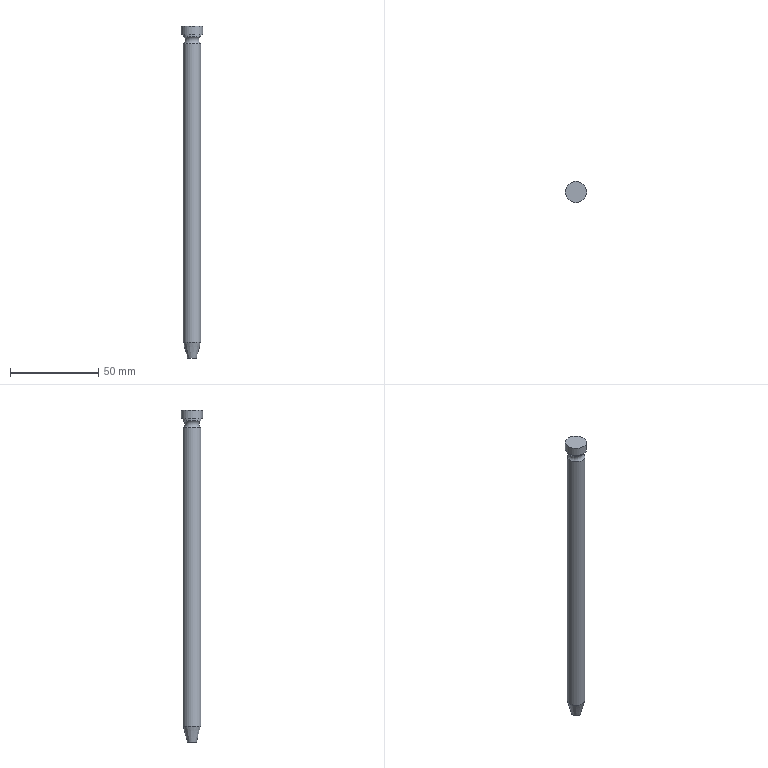Part | NX | features SMAL10-100-P9.97_1 2 | 1 solid | 8 faces | box 12 x 12 x 188 mm | volume 14568 mm3 | cylinder 3 | plane 3 | cone 1 | torus 1 | commonest cylinder face diameters 10 x2 12 x1
STEP:
#1=CARTESIAN_POINT('',(275.029,-406.95,85.95));
#2=VERTEX_POINT('',#1);
#3=CARTESIAN_POINT('',(275.029,-411.95,85.95));
#4=DIRECTION('',(0.,0.,-1.));
#5=DIRECTION('',(0.,1.,0.));
#6=AXIS2_PLACEMENT_3D('',#3,#4,#5);
#7=CIRCLE('',#6,5.);
#8=EDGE_CURVE('',#2,#2,#7,.T.);
#9=ORIENTED_EDGE('',*,*,#8,.T.);
#10=EDGE_LOOP('',(#9));
#11=FACE_BOUND('',#10,.T.);
#12=CARTESIAN_POINT('',(275.029,-416.95,-82.894));
#13=VERTEX_POINT('',#12);
#14=CARTESIAN_POINT('',(275.029,-411.95,-82.894));
#15=DIRECTION('',(0.,0.,-1.));
#16=DIRECTION('',(0.,-1.,0.));
#17=AXIS2_PLACEMENT_3D('',#14,#15,#16);
#18=CIRCLE('',#17,5.);
#19=EDGE_CURVE('',#13,#13,#18,.T.);
#20=ORIENTED_EDGE('',*,*,#19,.F.);
#21=EDGE_LOOP('',(#20));
#22=FACE_BOUND('',#21,.T.);
#23=CARTESIAN_POINT('',(275.029,-411.95,51.55));
#24=DIRECTION('',(0.,0.,-1.));
#25=DIRECTION('',(0.,1.,0.));
#26=AXIS2_PLACEMENT_3D('',#23,#24,#25);
#27=CYLINDRICAL_SURFACE('',#26,5.);
#28=ADVANCED_FACE('',(#11,#22),#27,.T.);
#29=ORIENTED_EDGE('',*,*,#19,.T.);
#30=EDGE_LOOP('',(#29));
#31=FACE_BOUND('',#30,.T.);
#32=CARTESIAN_POINT('',(275.029,-409.377,-91.95));
#33=VERTEX_POINT('',#32);
#34=CARTESIAN_POINT('',(275.029,-411.95,-91.95));
#35=DIRECTION('',(0.,0.,1.));
#36=DIRECTION('',(0.,1.,0.));
#37=AXIS2_PLACEMENT_3D('',#34,#35,#36);
#38=CIRCLE('',#37,2.573);
#39=EDGE_CURVE('',#33,#33,#38,.T.);
#40=ORIENTED_EDGE('',*,*,#39,.T.);
#41=EDGE_LOOP('',(#40));
#42=FACE_BOUND('',#41,.T.);
#43=CARTESIAN_POINT('',(275.029,-411.95,-85.95));
#44=DIRECTION('',(0.,0.,1.));
#45=DIRECTION('',(0.,-1.,0.));
#46=AXIS2_PLACEMENT_3D('',#43,#44,#45);
#47=CONICAL_SURFACE('',#46,4.181,0.2618);
#48=ADVANCED_FACE('',(#31,#42),#47,.T.);
#49=ORIENTED_EDGE('',*,*,#39,.F.);
#50=EDGE_LOOP('',(#49));
#51=FACE_BOUND('',#50,.T.);
#52=CARTESIAN_POINT('',(275.029,-411.95,-91.95));
#53=DIRECTION('',(0.,0.,-1.));
#54=DIRECTION('',(0.,1.,0.));
#55=AXIS2_PLACEMENT_3D('',#52,#53,#54);
#56=PLANE('',#55);
#57=ADVANCED_FACE('',(#51),#56,.T.);
#58=ORIENTED_EDGE('',*,*,#8,.F.);
#59=EDGE_LOOP('',(#58));
#60=FACE_BOUND('',#59,.T.);
#61=CARTESIAN_POINT('',(275.029,-406.95,89.95));
#62=VERTEX_POINT('',#61);
#63=CARTESIAN_POINT('',(275.029,-411.95,89.95));
#64=DIRECTION('',(0.,0.,1.));
#65=DIRECTION('',(0.,1.,0.));
#66=AXIS2_PLACEMENT_3D('',#63,#64,#65);
#67=CIRCLE('',#66,5.);
#68=EDGE_CURVE('',#62,#62,#67,.T.);
#69=ORIENTED_EDGE('',*,*,#68,.F.);
#70=EDGE_LOOP('',(#69));
#71=FACE_BOUND('',#70,.T.);
#72=CARTESIAN_POINT('',(275.029,-411.95,87.95));
#73=DIRECTION('',(0.,0.,-1.));
#74=DIRECTION('',(0.,1.,0.));
#75=AXIS2_PLACEMENT_3D('',#72,#73,#74);
#76=TOROIDAL_SURFACE('',#75,6.5,2.5);
#77=ADVANCED_FACE('',(#60,#71),#76,.F.);
#78=ORIENTED_EDGE('',*,*,#68,.T.);
#79=EDGE_LOOP('',(#78));
#80=FACE_BOUND('',#79,.T.);
#81=CARTESIAN_POINT('',(275.029,-406.95,91.05));
#82=VERTEX_POINT('',#81);
#83=CARTESIAN_POINT('',(275.029,-411.95,91.05));
#84=DIRECTION('',(0.,0.,1.));
#85=DIRECTION('',(0.,1.,0.));
#86=AXIS2_PLACEMENT_3D('',#83,#84,#85);
#87=CIRCLE('',#86,5.);
#88=EDGE_CURVE('',#82,#82,#87,.T.);
#89=ORIENTED_EDGE('',*,*,#88,.F.);
#90=EDGE_LOOP('',(#89));
#91=FACE_BOUND('',#90,.T.);
#92=CARTESIAN_POINT('',(275.029,-411.95,51.55));
#93=DIRECTION('',(0.,0.,-1.));
#94=DIRECTION('',(0.,1.,0.));
#95=AXIS2_PLACEMENT_3D('',#92,#93,#94);
#96=CYLINDRICAL_SURFACE('',#95,5.);
#97=ADVANCED_FACE('',(#80,#91),#96,.T.);
#98=CARTESIAN_POINT('',(275.029,-405.95,96.05));
#99=VERTEX_POINT('',#98);
#100=CARTESIAN_POINT('',(275.029,-411.95,96.05));
#101=DIRECTION('',(0.,0.,1.));
#102=DIRECTION('',(0.,1.,0.));
#103=AXIS2_PLACEMENT_3D('',#100,#101,#102);
#104=CIRCLE('',#103,6.);
#105=EDGE_CURVE('',#99,#99,#104,.T.);
#106=ORIENTED_EDGE('',*,*,#105,.F.);
#107=EDGE_LOOP('',(#106));
#108=FACE_BOUND('',#107,.T.);
#109=CARTESIAN_POINT('',(275.029,-405.95,91.05));
#110=VERTEX_POINT('',#109);
#111=CARTESIAN_POINT('',(275.029,-411.95,91.05));
#112=DIRECTION('',(0.,0.,-1.));
#113=DIRECTION('',(0.,1.,0.));
#114=AXIS2_PLACEMENT_3D('',#111,#112,#113);
#115=CIRCLE('',#114,6.);
#116=EDGE_CURVE('',#110,#110,#115,.T.);
#117=ORIENTED_EDGE('',*,*,#116,.F.);
#118=EDGE_LOOP('',(#117));
#119=FACE_BOUND('',#118,.T.);
#120=CARTESIAN_POINT('',(275.029,-411.95,93.55));
#121=DIRECTION('',(0.,0.,-1.));
#122=DIRECTION('',(0.,1.,0.));
#123=AXIS2_PLACEMENT_3D('',#120,#121,#122);
#124=CYLINDRICAL_SURFACE('',#123,6.);
#125=ADVANCED_FACE('',(#108,#119),#124,.T.);
#126=ORIENTED_EDGE('',*,*,#105,.T.);
#127=EDGE_LOOP('',(#126));
#128=FACE_BOUND('',#127,.T.);
#129=CARTESIAN_POINT('',(275.029,-411.95,96.05));
#130=DIRECTION('',(0.,0.,1.));
#131=DIRECTION('',(0.,-1.,0.));
#132=AXIS2_PLACEMENT_3D('',#129,#130,#131);
#133=PLANE('',#132);
#134=ADVANCED_FACE('',(#128),#133,.T.);
#135=ORIENTED_EDGE('',*,*,#88,.T.);
#136=EDGE_LOOP('',(#135));
#137=FACE_BOUND('',#136,.T.);
#138=ORIENTED_EDGE('',*,*,#116,.T.);
#139=EDGE_LOOP('',(#138));
#140=FACE_BOUND('',#139,.T.);
#141=CARTESIAN_POINT('',(275.029,-411.95,91.05));
#142=DIRECTION('',(0.,0.,-1.));
#143=DIRECTION('',(0.,1.,0.));
#144=AXIS2_PLACEMENT_3D('',#141,#142,#143);
#145=PLANE('',#144);
#146=ADVANCED_FACE('',(#137,#140),#145,.T.);
#147=CLOSED_SHELL('',(#28,#48,#57,#77,#97,#125,#134,#146));
#148=MANIFOLD_SOLID_BREP('',#147);
#149=(LENGTH_UNIT()NAMED_UNIT(*)SI_UNIT(.MILLI.,.METRE.));
#150=UNCERTAINTY_MEASURE_WITH_UNIT(LENGTH_MEASURE(0.00001),#149,'','');
#151=(NAMED_UNIT(*)PLANE_ANGLE_UNIT()SI_UNIT($,.RADIAN.));
#152=(NAMED_UNIT(*)SI_UNIT($,.STERADIAN.)SOLID_ANGLE_UNIT());
#153=(GEOMETRIC_REPRESENTATION_CONTEXT(3)GLOBAL_UNCERTAINTY_ASSIGNED_CONTEXT((#150))GLOBAL_UNIT_ASSIGNED_CONTEXT((#149,#151,#152))REPRESENTATION_CONTEXT('',''));
#154=ADVANCED_BREP_SHAPE_REPRESENTATION('',(#148),#153);